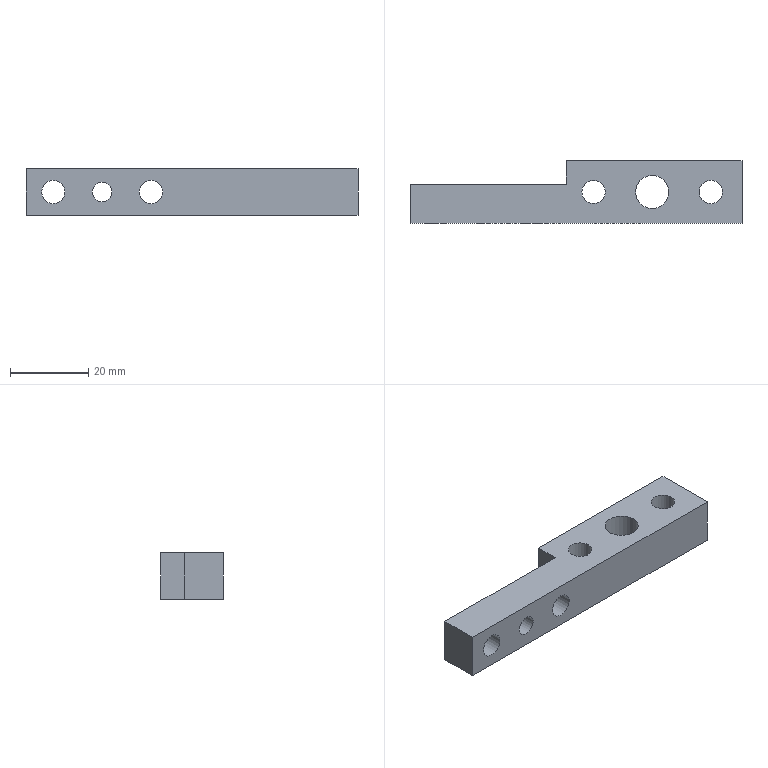Part | NX | features BREP 1 | 1 solid | 14 faces | box 85 x 16 x 12 mm | volume 11319 mm3 | plane 8 | cylinder 6 | commonest cylinder face diameters 6 x4 5 x1 8.5 x1
STEP:
#1=CARTESIAN_POINT('',(42.5,-8.,-6.));
#2=VERTEX_POINT('',#1);
#3=CARTESIAN_POINT('',(42.5,8.,-6.));
#4=VERTEX_POINT('',#3);
#5=CARTESIAN_POINT('',(42.5,-8.,-6.));
#6=DIRECTION('',(0.,1.,0.));
#7=VECTOR('',#6,1000.);
#8=LINE('',#5,#7);
#9=EDGE_CURVE('',#2,#4,#8,.T.);
#10=ORIENTED_EDGE('',*,*,#9,.T.);
#11=CARTESIAN_POINT('',(42.5,8.,6.));
#12=VERTEX_POINT('',#11);
#13=CARTESIAN_POINT('',(42.5,8.,6.));
#14=DIRECTION('',(0.,0.,-1.));
#15=VECTOR('',#14,1000.);
#16=LINE('',#13,#15);
#17=EDGE_CURVE('',#12,#4,#16,.T.);
#18=ORIENTED_EDGE('',*,*,#17,.F.);
#19=CARTESIAN_POINT('',(42.5,-8.,6.));
#20=VERTEX_POINT('',#19);
#21=CARTESIAN_POINT('',(42.5,-8.,6.));
#22=DIRECTION('',(0.,1.,0.));
#23=VECTOR('',#22,1000.);
#24=LINE('',#21,#23);
#25=EDGE_CURVE('',#20,#12,#24,.T.);
#26=ORIENTED_EDGE('',*,*,#25,.F.);
#27=CARTESIAN_POINT('',(42.5,-8.,6.));
#28=DIRECTION('',(0.,0.,-1.));
#29=VECTOR('',#28,1000.);
#30=LINE('',#27,#29);
#31=EDGE_CURVE('',#20,#2,#30,.T.);
#32=ORIENTED_EDGE('',*,*,#31,.T.);
#33=EDGE_LOOP('',(#10,#18,#26,#32));
#34=FACE_BOUND('',#33,.T.);
#35=CARTESIAN_POINT('',(42.5,-8.,6.));
#36=DIRECTION('',(-1.,0.,0.));
#37=DIRECTION('',(0.,0.,-1.));
#38=AXIS2_PLACEMENT_3D('',#35,#36,#37);
#39=PLANE('',#38);
#40=ADVANCED_FACE('',(#34),#39,.F.);
#41=CARTESIAN_POINT('',(-2.5,8.,-6.));
#42=VERTEX_POINT('',#41);
#43=CARTESIAN_POINT('',(-42.5,8.,-6.));
#44=DIRECTION('',(-1.,0.,0.));
#45=VECTOR('',#44,1000.);
#46=LINE('',#43,#45);
#47=EDGE_CURVE('',#4,#42,#46,.T.);
#48=ORIENTED_EDGE('',*,*,#47,.T.);
#49=CARTESIAN_POINT('',(-2.5,8.,6.));
#50=VERTEX_POINT('',#49);
#51=CARTESIAN_POINT('',(-2.5,8.,-46.447));
#52=DIRECTION('',(0.,0.,1.));
#53=VECTOR('',#52,1000.);
#54=LINE('',#51,#53);
#55=EDGE_CURVE('',#42,#50,#54,.T.);
#56=ORIENTED_EDGE('',*,*,#55,.T.);
#57=CARTESIAN_POINT('',(-42.5,8.,6.));
#58=DIRECTION('',(-1.,0.,0.));
#59=VECTOR('',#58,1000.);
#60=LINE('',#57,#59);
#61=EDGE_CURVE('',#12,#50,#60,.T.);
#62=ORIENTED_EDGE('',*,*,#61,.F.);
#63=ORIENTED_EDGE('',*,*,#17,.T.);
#64=EDGE_LOOP('',(#48,#56,#62,#63));
#65=FACE_BOUND('',#64,.T.);
#66=CARTESIAN_POINT('',(-42.5,8.,6.));
#67=DIRECTION('',(0.,-1.,0.));
#68=DIRECTION('',(0.,0.,1.));
#69=AXIS2_PLACEMENT_3D('',#66,#67,#68);
#70=PLANE('',#69);
#71=ADVANCED_FACE('',(#65),#70,.F.);
#72=CARTESIAN_POINT('',(-42.5,2.,6.));
#73=VERTEX_POINT('',#72);
#74=CARTESIAN_POINT('',(-42.5,-8.,6.));
#75=VERTEX_POINT('',#74);
#76=CARTESIAN_POINT('',(-42.5,-8.,6.));
#77=DIRECTION('',(0.,-1.,0.));
#78=VECTOR('',#77,1000.);
#79=LINE('',#76,#78);
#80=EDGE_CURVE('',#73,#75,#79,.T.);
#81=ORIENTED_EDGE('',*,*,#80,.F.);
#82=CARTESIAN_POINT('',(-42.5,2.,-6.));
#83=VERTEX_POINT('',#82);
#84=CARTESIAN_POINT('',(-42.5,2.,-46.447));
#85=DIRECTION('',(0.,0.,1.));
#86=VECTOR('',#85,1000.);
#87=LINE('',#84,#86);
#88=EDGE_CURVE('',#83,#73,#87,.T.);
#89=ORIENTED_EDGE('',*,*,#88,.F.);
#90=CARTESIAN_POINT('',(-42.5,-8.,-6.));
#91=VERTEX_POINT('',#90);
#92=CARTESIAN_POINT('',(-42.5,-8.,-6.));
#93=DIRECTION('',(0.,-1.,0.));
#94=VECTOR('',#93,1000.);
#95=LINE('',#92,#94);
#96=EDGE_CURVE('',#83,#91,#95,.T.);
#97=ORIENTED_EDGE('',*,*,#96,.T.);
#98=CARTESIAN_POINT('',(-42.5,-8.,6.));
#99=DIRECTION('',(0.,0.,-1.));
#100=VECTOR('',#99,1000.);
#101=LINE('',#98,#100);
#102=EDGE_CURVE('',#75,#91,#101,.T.);
#103=ORIENTED_EDGE('',*,*,#102,.F.);
#104=EDGE_LOOP('',(#81,#89,#97,#103));
#105=FACE_BOUND('',#104,.T.);
#106=CARTESIAN_POINT('',(-42.5,-8.,6.));
#107=DIRECTION('',(1.,0.,0.));
#108=DIRECTION('',(0.,0.,1.));
#109=AXIS2_PLACEMENT_3D('',#106,#107,#108);
#110=PLANE('',#109);
#111=ADVANCED_FACE('',(#105),#110,.F.);
#112=CARTESIAN_POINT('',(-23.,-8.,2.5));
#113=VERTEX_POINT('',#112);
#114=CARTESIAN_POINT('',(-23.,-8.,0.));
#115=DIRECTION('',(0.,1.,0.));
#116=DIRECTION('',(0.,0.,1.));
#117=AXIS2_PLACEMENT_3D('',#114,#115,#116);
#118=CIRCLE('',#117,2.5);
#119=EDGE_CURVE('',#113,#113,#118,.T.);
#120=ORIENTED_EDGE('',*,*,#119,.T.);
#121=EDGE_LOOP('',(#120));
#122=FACE_BOUND('',#121,.T.);
#123=CARTESIAN_POINT('',(-10.5,-8.,3.));
#124=VERTEX_POINT('',#123);
#125=CARTESIAN_POINT('',(-10.5,-8.,0.));
#126=DIRECTION('',(0.,1.,0.));
#127=DIRECTION('',(0.,0.,1.));
#128=AXIS2_PLACEMENT_3D('',#125,#126,#127);
#129=CIRCLE('',#128,3.);
#130=EDGE_CURVE('',#124,#124,#129,.T.);
#131=ORIENTED_EDGE('',*,*,#130,.T.);
#132=EDGE_LOOP('',(#131));
#133=FACE_BOUND('',#132,.T.);
#134=CARTESIAN_POINT('',(-35.5,-8.,3.));
#135=VERTEX_POINT('',#134);
#136=CARTESIAN_POINT('',(-35.5,-8.,0.));
#137=DIRECTION('',(0.,1.,0.));
#138=DIRECTION('',(0.,0.,1.));
#139=AXIS2_PLACEMENT_3D('',#136,#137,#138);
#140=CIRCLE('',#139,3.);
#141=EDGE_CURVE('',#135,#135,#140,.T.);
#142=ORIENTED_EDGE('',*,*,#141,.T.);
#143=EDGE_LOOP('',(#142));
#144=FACE_BOUND('',#143,.T.);
#145=CARTESIAN_POINT('',(-42.5,-8.,-6.));
#146=DIRECTION('',(1.,0.,0.));
#147=VECTOR('',#146,1000.);
#148=LINE('',#145,#147);
#149=EDGE_CURVE('',#91,#2,#148,.T.);
#150=ORIENTED_EDGE('',*,*,#149,.T.);
#151=ORIENTED_EDGE('',*,*,#31,.F.);
#152=CARTESIAN_POINT('',(-42.5,-8.,6.));
#153=DIRECTION('',(1.,0.,0.));
#154=VECTOR('',#153,1000.);
#155=LINE('',#152,#154);
#156=EDGE_CURVE('',#75,#20,#155,.T.);
#157=ORIENTED_EDGE('',*,*,#156,.F.);
#158=ORIENTED_EDGE('',*,*,#102,.T.);
#159=EDGE_LOOP('',(#150,#151,#157,#158));
#160=FACE_BOUND('',#159,.T.);
#161=CARTESIAN_POINT('',(-42.5,-8.,6.));
#162=DIRECTION('',(0.,1.,0.));
#163=DIRECTION('',(0.,0.,-1.));
#164=AXIS2_PLACEMENT_3D('',#161,#162,#163);
#165=PLANE('',#164);
#166=ADVANCED_FACE('',(#122,#133,#144,#160),#165,.F.);
#167=CARTESIAN_POINT('',(23.75,0.,6.));
#168=VERTEX_POINT('',#167);
#169=CARTESIAN_POINT('',(19.5,0.,6.));
#170=DIRECTION('',(0.,0.,1.));
#171=DIRECTION('',(1.,0.,0.));
#172=AXIS2_PLACEMENT_3D('',#169,#170,#171);
#173=CIRCLE('',#172,4.25);
#174=EDGE_CURVE('',#168,#168,#173,.T.);
#175=ORIENTED_EDGE('',*,*,#174,.F.);
#176=EDGE_LOOP('',(#175));
#177=FACE_BOUND('',#176,.T.);
#178=CARTESIAN_POINT('',(37.5,0.,6.));
#179=VERTEX_POINT('',#178);
#180=CARTESIAN_POINT('',(34.5,0.,6.));
#181=DIRECTION('',(0.,0.,1.));
#182=DIRECTION('',(1.,0.,0.));
#183=AXIS2_PLACEMENT_3D('',#180,#181,#182);
#184=CIRCLE('',#183,3.);
#185=EDGE_CURVE('',#179,#179,#184,.T.);
#186=ORIENTED_EDGE('',*,*,#185,.F.);
#187=EDGE_LOOP('',(#186));
#188=FACE_BOUND('',#187,.T.);
#189=CARTESIAN_POINT('',(7.5,0.,6.));
#190=VERTEX_POINT('',#189);
#191=CARTESIAN_POINT('',(4.5,0.,6.));
#192=DIRECTION('',(0.,0.,1.));
#193=DIRECTION('',(1.,0.,0.));
#194=AXIS2_PLACEMENT_3D('',#191,#192,#193);
#195=CIRCLE('',#194,3.);
#196=EDGE_CURVE('',#190,#190,#195,.T.);
#197=ORIENTED_EDGE('',*,*,#196,.F.);
#198=EDGE_LOOP('',(#197));
#199=FACE_BOUND('',#198,.T.);
#200=CARTESIAN_POINT('',(-2.5,2.,6.));
#201=VERTEX_POINT('',#200);
#202=CARTESIAN_POINT('',(-2.5,8.,6.));
#203=DIRECTION('',(0.,1.,0.));
#204=VECTOR('',#203,1000.);
#205=LINE('',#202,#204);
#206=EDGE_CURVE('',#201,#50,#205,.T.);
#207=ORIENTED_EDGE('',*,*,#206,.F.);
#208=CARTESIAN_POINT('',(-42.5,2.,6.));
#209=DIRECTION('',(1.,0.,0.));
#210=VECTOR('',#209,1000.);
#211=LINE('',#208,#210);
#212=EDGE_CURVE('',#73,#201,#211,.T.);
#213=ORIENTED_EDGE('',*,*,#212,.F.);
#214=ORIENTED_EDGE('',*,*,#80,.T.);
#215=ORIENTED_EDGE('',*,*,#156,.T.);
#216=ORIENTED_EDGE('',*,*,#25,.T.);
#217=ORIENTED_EDGE('',*,*,#61,.T.);
#218=EDGE_LOOP('',(#207,#213,#214,#215,#216,#217));
#219=FACE_BOUND('',#218,.T.);
#220=CARTESIAN_POINT('',(0.,0.,6.));
#221=DIRECTION('',(0.,0.,-1.));
#222=DIRECTION('',(1.,0.,0.));
#223=AXIS2_PLACEMENT_3D('',#220,#221,#222);
#224=PLANE('',#223);
#225=ADVANCED_FACE('',(#177,#188,#199,#219),#224,.F.);
#226=CARTESIAN_POINT('',(-2.5,2.,-6.));
#227=VERTEX_POINT('',#226);
#228=CARTESIAN_POINT('',(-42.5,2.,-6.));
#229=DIRECTION('',(1.,0.,0.));
#230=VECTOR('',#229,1000.);
#231=LINE('',#228,#230);
#232=EDGE_CURVE('',#83,#227,#231,.T.);
#233=ORIENTED_EDGE('',*,*,#232,.T.);
#234=CARTESIAN_POINT('',(-2.5,8.,-6.));
#235=DIRECTION('',(0.,1.,0.));
#236=VECTOR('',#235,1000.);
#237=LINE('',#234,#236);
#238=EDGE_CURVE('',#227,#42,#237,.T.);
#239=ORIENTED_EDGE('',*,*,#238,.T.);
#240=ORIENTED_EDGE('',*,*,#47,.F.);
#241=ORIENTED_EDGE('',*,*,#9,.F.);
#242=ORIENTED_EDGE('',*,*,#149,.F.);
#243=ORIENTED_EDGE('',*,*,#96,.F.);
#244=EDGE_LOOP('',(#233,#239,#240,#241,#242,#243));
#245=FACE_BOUND('',#244,.T.);
#246=CARTESIAN_POINT('',(23.75,0.,-6.));
#247=VERTEX_POINT('',#246);
#248=CARTESIAN_POINT('',(19.5,0.,-6.));
#249=DIRECTION('',(0.,0.,1.));
#250=DIRECTION('',(1.,0.,0.));
#251=AXIS2_PLACEMENT_3D('',#248,#249,#250);
#252=CIRCLE('',#251,4.25);
#253=EDGE_CURVE('',#247,#247,#252,.T.);
#254=ORIENTED_EDGE('',*,*,#253,.T.);
#255=EDGE_LOOP('',(#254));
#256=FACE_BOUND('',#255,.T.);
#257=CARTESIAN_POINT('',(37.5,0.,-6.));
#258=VERTEX_POINT('',#257);
#259=CARTESIAN_POINT('',(34.5,0.,-6.));
#260=DIRECTION('',(0.,0.,1.));
#261=DIRECTION('',(1.,0.,0.));
#262=AXIS2_PLACEMENT_3D('',#259,#260,#261);
#263=CIRCLE('',#262,3.);
#264=EDGE_CURVE('',#258,#258,#263,.T.);
#265=ORIENTED_EDGE('',*,*,#264,.T.);
#266=EDGE_LOOP('',(#265));
#267=FACE_BOUND('',#266,.T.);
#268=CARTESIAN_POINT('',(7.5,0.,-6.));
#269=VERTEX_POINT('',#268);
#270=CARTESIAN_POINT('',(4.5,0.,-6.));
#271=DIRECTION('',(0.,0.,1.));
#272=DIRECTION('',(1.,0.,0.));
#273=AXIS2_PLACEMENT_3D('',#270,#271,#272);
#274=CIRCLE('',#273,3.);
#275=EDGE_CURVE('',#269,#269,#274,.T.);
#276=ORIENTED_EDGE('',*,*,#275,.T.);
#277=EDGE_LOOP('',(#276));
#278=FACE_BOUND('',#277,.T.);
#279=CARTESIAN_POINT('',(0.,0.,-6.));
#280=DIRECTION('',(0.,0.,-1.));
#281=DIRECTION('',(1.,0.,0.));
#282=AXIS2_PLACEMENT_3D('',#279,#280,#281);
#283=PLANE('',#282);
#284=ADVANCED_FACE('',(#245,#256,#267,#278),#283,.T.);
#285=ORIENTED_EDGE('',*,*,#275,.F.);
#286=EDGE_LOOP('',(#285));
#287=FACE_BOUND('',#286,.T.);
#288=ORIENTED_EDGE('',*,*,#196,.T.);
#289=EDGE_LOOP('',(#288));
#290=FACE_BOUND('',#289,.T.);
#291=CARTESIAN_POINT('',(4.5,0.,6.));
#292=DIRECTION('',(0.,0.,1.));
#293=DIRECTION('',(-1.,0.,0.));
#294=AXIS2_PLACEMENT_3D('',#291,#292,#293);
#295=CYLINDRICAL_SURFACE('',#294,3.);
#296=ADVANCED_FACE('',(#287,#290),#295,.F.);
#297=ORIENTED_EDGE('',*,*,#264,.F.);
#298=EDGE_LOOP('',(#297));
#299=FACE_BOUND('',#298,.T.);
#300=ORIENTED_EDGE('',*,*,#185,.T.);
#301=EDGE_LOOP('',(#300));
#302=FACE_BOUND('',#301,.T.);
#303=CARTESIAN_POINT('',(34.5,0.,6.));
#304=DIRECTION('',(0.,0.,1.));
#305=DIRECTION('',(-1.,0.,0.));
#306=AXIS2_PLACEMENT_3D('',#303,#304,#305);
#307=CYLINDRICAL_SURFACE('',#306,3.);
#308=ADVANCED_FACE('',(#299,#302),#307,.F.);
#309=ORIENTED_EDGE('',*,*,#253,.F.);
#310=EDGE_LOOP('',(#309));
#311=FACE_BOUND('',#310,.T.);
#312=ORIENTED_EDGE('',*,*,#174,.T.);
#313=EDGE_LOOP('',(#312));
#314=FACE_BOUND('',#313,.T.);
#315=CARTESIAN_POINT('',(19.5,0.,6.));
#316=DIRECTION('',(0.,0.,1.));
#317=DIRECTION('',(-1.,0.,0.));
#318=AXIS2_PLACEMENT_3D('',#315,#316,#317);
#319=CYLINDRICAL_SURFACE('',#318,4.25);
#320=ADVANCED_FACE('',(#311,#314),#319,.F.);
#321=CARTESIAN_POINT('',(-23.,2.,2.5));
#322=VERTEX_POINT('',#321);
#323=CARTESIAN_POINT('',(-23.,2.,0.));
#324=DIRECTION('',(0.,1.,0.));
#325=DIRECTION('',(0.,0.,1.));
#326=AXIS2_PLACEMENT_3D('',#323,#324,#325);
#327=CIRCLE('',#326,2.5);
#328=EDGE_CURVE('',#322,#322,#327,.T.);
#329=ORIENTED_EDGE('',*,*,#328,.F.);
#330=EDGE_LOOP('',(#329));
#331=FACE_BOUND('',#330,.T.);
#332=CARTESIAN_POINT('',(-10.5,2.,3.));
#333=VERTEX_POINT('',#332);
#334=CARTESIAN_POINT('',(-10.5,2.,0.));
#335=DIRECTION('',(0.,1.,0.));
#336=DIRECTION('',(0.,0.,1.));
#337=AXIS2_PLACEMENT_3D('',#334,#335,#336);
#338=CIRCLE('',#337,3.);
#339=EDGE_CURVE('',#333,#333,#338,.T.);
#340=ORIENTED_EDGE('',*,*,#339,.F.);
#341=EDGE_LOOP('',(#340));
#342=FACE_BOUND('',#341,.T.);
#343=CARTESIAN_POINT('',(-35.5,2.,3.));
#344=VERTEX_POINT('',#343);
#345=CARTESIAN_POINT('',(-35.5,2.,0.));
#346=DIRECTION('',(0.,1.,0.));
#347=DIRECTION('',(0.,0.,1.));
#348=AXIS2_PLACEMENT_3D('',#345,#346,#347);
#349=CIRCLE('',#348,3.);
#350=EDGE_CURVE('',#344,#344,#349,.T.);
#351=ORIENTED_EDGE('',*,*,#350,.F.);
#352=EDGE_LOOP('',(#351));
#353=FACE_BOUND('',#352,.T.);
#354=ORIENTED_EDGE('',*,*,#88,.T.);
#355=ORIENTED_EDGE('',*,*,#212,.T.);
#356=CARTESIAN_POINT('',(-2.5,2.,-46.447));
#357=DIRECTION('',(0.,0.,1.));
#358=VECTOR('',#357,1000.);
#359=LINE('',#356,#358);
#360=EDGE_CURVE('',#227,#201,#359,.T.);
#361=ORIENTED_EDGE('',*,*,#360,.F.);
#362=ORIENTED_EDGE('',*,*,#232,.F.);
#363=EDGE_LOOP('',(#354,#355,#361,#362));
#364=FACE_BOUND('',#363,.T.);
#365=CARTESIAN_POINT('',(-42.5,2.,-46.447));
#366=DIRECTION('',(0.,-1.,0.));
#367=DIRECTION('',(0.,0.,1.));
#368=AXIS2_PLACEMENT_3D('',#365,#366,#367);
#369=PLANE('',#368);
#370=ADVANCED_FACE('',(#331,#342,#353,#364),#369,.F.);
#371=ORIENTED_EDGE('',*,*,#360,.T.);
#372=ORIENTED_EDGE('',*,*,#206,.T.);
#373=ORIENTED_EDGE('',*,*,#55,.F.);
#374=ORIENTED_EDGE('',*,*,#238,.F.);
#375=EDGE_LOOP('',(#371,#372,#373,#374));
#376=FACE_BOUND('',#375,.T.);
#377=CARTESIAN_POINT('',(-2.5,8.,-46.447));
#378=DIRECTION('',(1.,0.,0.));
#379=DIRECTION('',(0.,0.,1.));
#380=AXIS2_PLACEMENT_3D('',#377,#378,#379);
#381=PLANE('',#380);
#382=ADVANCED_FACE('',(#376),#381,.F.);
#383=ORIENTED_EDGE('',*,*,#141,.F.);
#384=EDGE_LOOP('',(#383));
#385=FACE_BOUND('',#384,.T.);
#386=ORIENTED_EDGE('',*,*,#350,.T.);
#387=EDGE_LOOP('',(#386));
#388=FACE_BOUND('',#387,.T.);
#389=CARTESIAN_POINT('',(-35.5,2.,0.));
#390=DIRECTION('',(0.,1.,0.));
#391=DIRECTION('',(0.,0.,-1.));
#392=AXIS2_PLACEMENT_3D('',#389,#390,#391);
#393=CYLINDRICAL_SURFACE('',#392,3.);
#394=ADVANCED_FACE('',(#385,#388),#393,.F.);
#395=ORIENTED_EDGE('',*,*,#130,.F.);
#396=EDGE_LOOP('',(#395));
#397=FACE_BOUND('',#396,.T.);
#398=ORIENTED_EDGE('',*,*,#339,.T.);
#399=EDGE_LOOP('',(#398));
#400=FACE_BOUND('',#399,.T.);
#401=CARTESIAN_POINT('',(-10.5,2.,0.));
#402=DIRECTION('',(0.,1.,0.));
#403=DIRECTION('',(0.,0.,-1.));
#404=AXIS2_PLACEMENT_3D('',#401,#402,#403);
#405=CYLINDRICAL_SURFACE('',#404,3.);
#406=ADVANCED_FACE('',(#397,#400),#405,.F.);
#407=ORIENTED_EDGE('',*,*,#119,.F.);
#408=EDGE_LOOP('',(#407));
#409=FACE_BOUND('',#408,.T.);
#410=ORIENTED_EDGE('',*,*,#328,.T.);
#411=EDGE_LOOP('',(#410));
#412=FACE_BOUND('',#411,.T.);
#413=CARTESIAN_POINT('',(-23.,2.,0.));
#414=DIRECTION('',(0.,1.,0.));
#415=DIRECTION('',(0.,0.,-1.));
#416=AXIS2_PLACEMENT_3D('',#413,#414,#415);
#417=CYLINDRICAL_SURFACE('',#416,2.5);
#418=ADVANCED_FACE('',(#409,#412),#417,.F.);
#419=CLOSED_SHELL('',(#40,#71,#111,#166,#225,#284,#296,#308,#320,#370,#382,#394,#406,#418));
#420=MANIFOLD_SOLID_BREP('',#419);
#421=(LENGTH_UNIT()NAMED_UNIT(*)SI_UNIT(.MILLI.,.METRE.));
#422=UNCERTAINTY_MEASURE_WITH_UNIT(LENGTH_MEASURE(0.00001),#421,'','');
#423=(NAMED_UNIT(*)PLANE_ANGLE_UNIT()SI_UNIT($,.RADIAN.));
#424=(NAMED_UNIT(*)SI_UNIT($,.STERADIAN.)SOLID_ANGLE_UNIT());
#425=(GEOMETRIC_REPRESENTATION_CONTEXT(3)GLOBAL_UNCERTAINTY_ASSIGNED_CONTEXT((#422))GLOBAL_UNIT_ASSIGNED_CONTEXT((#421,#423,#424))REPRESENTATION_CONTEXT('',''));
#426=ADVANCED_BREP_SHAPE_REPRESENTATION('',(#420),#425);